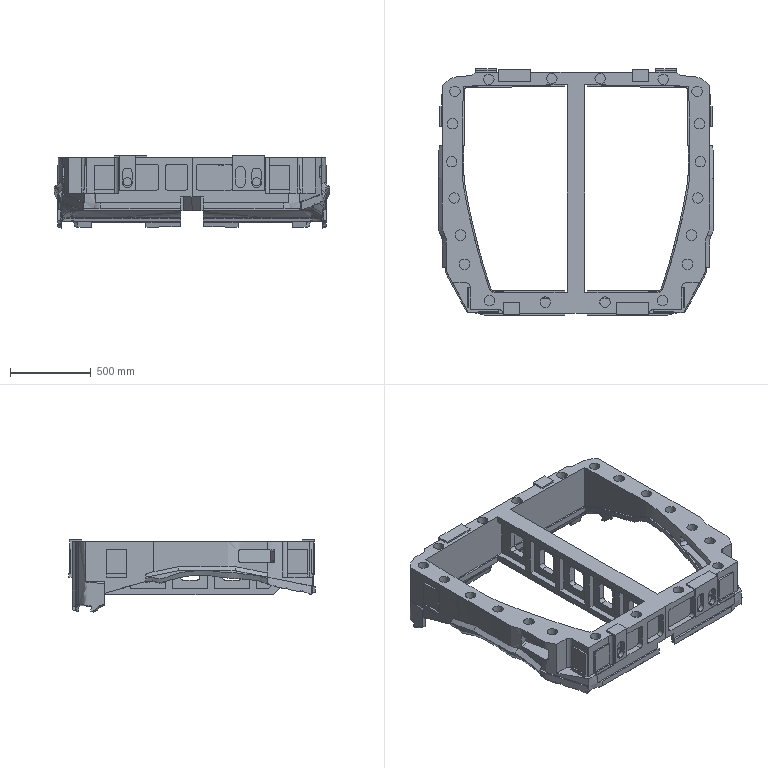Part | NX | features solid 2 | 1 solid | 952 faces | box 1704 x 1525 x 446.585 mm | volume 186102622 mm3 | spline 505 | plane 321 | cylinder 126 | commonest cylinder face diameters 40 x54 52 x28 65 x20 20 x8 10 x4 48 x4